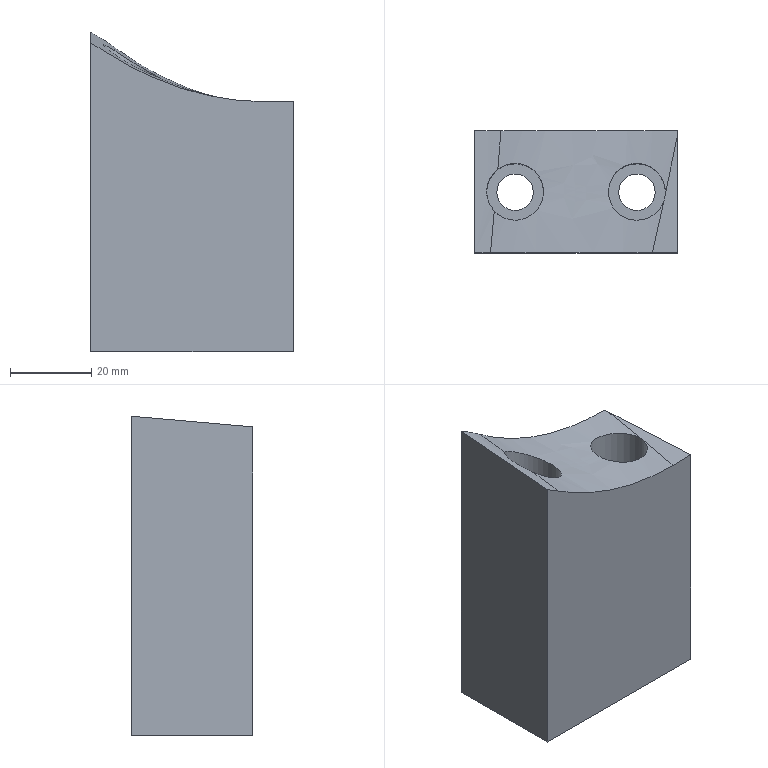Part | NX | features solid 2 | 1 solid | 14 faces | box 50.002 x 30 x 78.739 mm | volume 80442 mm3 | plane 7 | cylinder 4 | spline 3 | commonest cylinder face diameters 9 x2 14 x2
STEP:
#1=CARTESIAN_POINT('',(157.5,150.,-6.261));
#2=VERTEX_POINT('',#1);
#3=CARTESIAN_POINT('',(157.5,150.,-85.));
#4=VERTEX_POINT('',#3);
#5=CARTESIAN_POINT('',(157.5,150.,10.));
#6=DIRECTION('',(0.,0.,-1.));
#7=VECTOR('',#6,1000.);
#8=LINE('',#5,#7);
#9=EDGE_CURVE('',#2,#4,#8,.T.);
#10=ORIENTED_EDGE('',*,*,#9,.F.);
#11=CARTESIAN_POINT('',(164.005,150.,-10.429));
#12=VERTEX_POINT('',#11);
#13=CARTESIAN_POINT('',(157.5,150.,-6.261));
#14=CARTESIAN_POINT('',(159.786,150.,-7.489));
#15=CARTESIAN_POINT('',(161.955,150.,-8.881));
#16=CARTESIAN_POINT('',(164.008,150.,-10.435));
#17=B_SPLINE_CURVE_WITH_KNOTS('',3,(#13,#14,#15,#16),.UNSPECIFIED.,.F.,.F.,(4,4),(0.,0.007722),.UNSPECIFIED.);
#18=EDGE_CURVE('',#2,#12,#17,.T.);
#19=ORIENTED_EDGE('',*,*,#18,.T.);
#20=CARTESIAN_POINT('',(207.5,150.,-24.818));
#21=VERTEX_POINT('',#20);
#22=CARTESIAN_POINT('',(164.004,150.,-10.427));
#23=CARTESIAN_POINT('',(165.563,150.,-11.606));
#24=CARTESIAN_POINT('',(168.794,150.,-13.755));
#25=CARTESIAN_POINT('',(175.477,150.,-17.617));
#26=CARTESIAN_POINT('',(187.998,150.,-22.995));
#27=CARTESIAN_POINT('',(199.69,150.,-24.897));
#28=CARTESIAN_POINT('',(207.5,150.,-24.818));
#29=B_SPLINE_CURVE_WITH_KNOTS('',3,(#22,#23,#24,#25,#26,#27,#28),.UNSPECIFIED.,.F.,.F.,(4,1,1,1,4),(0.,0.00579,0.01158,0.02316,0.04632),.UNSPECIFIED.);
#30=EDGE_CURVE('',#12,#21,#29,.T.);
#31=ORIENTED_EDGE('',*,*,#30,.T.);
#32=CARTESIAN_POINT('',(207.5,150.,-85.));
#33=VERTEX_POINT('',#32);
#34=CARTESIAN_POINT('',(207.5,150.,10.));
#35=DIRECTION('',(0.,0.,-1.));
#36=VECTOR('',#35,1000.);
#37=LINE('',#34,#36);
#38=EDGE_CURVE('',#21,#33,#37,.T.);
#39=ORIENTED_EDGE('',*,*,#38,.T.);
#40=CARTESIAN_POINT('',(157.5,150.,-85.));
#41=DIRECTION('',(1.,0.,0.));
#42=VECTOR('',#41,1000.);
#43=LINE('',#40,#42);
#44=EDGE_CURVE('',#4,#33,#43,.T.);
#45=ORIENTED_EDGE('',*,*,#44,.F.);
#46=EDGE_LOOP('',(#10,#19,#31,#39,#45));
#47=FACE_BOUND('',#46,.T.);
#48=CARTESIAN_POINT('',(157.5,150.,10.));
#49=DIRECTION('',(0.,-1.,0.));
#50=DIRECTION('',(0.,0.,-1.));
#51=AXIS2_PLACEMENT_3D('',#48,#49,#50);
#52=PLANE('',#51);
#53=ADVANCED_FACE('',(#47),#52,.F.);
#54=CARTESIAN_POINT('',(207.5,120.,-23.313));
#55=VERTEX_POINT('',#54);
#56=CARTESIAN_POINT('',(207.5,120.,-85.));
#57=VERTEX_POINT('',#56);
#58=CARTESIAN_POINT('',(207.5,120.,10.));
#59=DIRECTION('',(0.,0.,-1.));
#60=VECTOR('',#59,1000.);
#61=LINE('',#58,#60);
#62=EDGE_CURVE('',#55,#57,#61,.T.);
#63=ORIENTED_EDGE('',*,*,#62,.F.);
#64=CARTESIAN_POINT('',(201.315,120.,-23.399));
#65=VERTEX_POINT('',#64);
#66=CARTESIAN_POINT('',(207.5,120.,-23.313));
#67=CARTESIAN_POINT('',(205.438,120.,-23.34));
#68=CARTESIAN_POINT('',(203.376,120.,-23.366));
#69=CARTESIAN_POINT('',(201.314,120.,-23.393));
#70=B_SPLINE_CURVE_WITH_KNOTS('',3,(#66,#67,#68,#69),.UNSPECIFIED.,.F.,.F.,(4,4),(0.,0.006187),.UNSPECIFIED.);
#71=EDGE_CURVE('',#55,#65,#70,.T.);
#72=ORIENTED_EDGE('',*,*,#71,.T.);
#73=CARTESIAN_POINT('',(161.435,120.,-11.237));
#74=VERTEX_POINT('',#73);
#75=CARTESIAN_POINT('',(201.315,120.,-23.401));
#76=CARTESIAN_POINT('',(194.24,120.,-23.492));
#77=CARTESIAN_POINT('',(183.7,120.,-21.839));
#78=CARTESIAN_POINT('',(172.184,120.,-17.245));
#79=CARTESIAN_POINT('',(165.954,120.,-13.988));
#80=CARTESIAN_POINT('',(162.91,120.,-12.213));
#81=CARTESIAN_POINT('',(161.434,120.,-11.237));
#82=B_SPLINE_CURVE_WITH_KNOTS('',3,(#75,#76,#77,#78,#79,#80,#81),.UNSPECIFIED.,.F.,.F.,(4,1,1,1,4),(0.,0.02111,0.03166,0.03694,0.04222),.UNSPECIFIED.);
#83=EDGE_CURVE('',#65,#74,#82,.T.);
#84=ORIENTED_EDGE('',*,*,#83,.T.);
#85=CARTESIAN_POINT('',(157.5,120.,-8.886));
#86=VERTEX_POINT('',#85);
#87=CARTESIAN_POINT('',(161.436,120.,-11.238));
#88=CARTESIAN_POINT('',(160.164,120.,-10.397));
#89=CARTESIAN_POINT('',(158.853,120.,-9.613));
#90=CARTESIAN_POINT('',(157.5,120.,-8.886));
#91=B_SPLINE_CURVE_WITH_KNOTS('',3,(#87,#88,#89,#90),.UNSPECIFIED.,.F.,.F.,(4,4),(0.008039,0.01261),.UNSPECIFIED.);
#92=EDGE_CURVE('',#74,#86,#91,.T.);
#93=ORIENTED_EDGE('',*,*,#92,.T.);
#94=CARTESIAN_POINT('',(157.5,120.,-85.));
#95=VERTEX_POINT('',#94);
#96=CARTESIAN_POINT('',(157.5,120.,10.));
#97=DIRECTION('',(0.,0.,-1.));
#98=VECTOR('',#97,1000.);
#99=LINE('',#96,#98);
#100=EDGE_CURVE('',#86,#95,#99,.T.);
#101=ORIENTED_EDGE('',*,*,#100,.T.);
#102=CARTESIAN_POINT('',(157.5,120.,-85.));
#103=DIRECTION('',(-1.,0.,0.));
#104=VECTOR('',#103,1000.);
#105=LINE('',#102,#104);
#106=EDGE_CURVE('',#95,#57,#105,.F.);
#107=ORIENTED_EDGE('',*,*,#106,.T.);
#108=EDGE_LOOP('',(#63,#72,#84,#93,#101,#107));
#109=FACE_BOUND('',#108,.T.);
#110=CARTESIAN_POINT('',(157.5,120.,10.));
#111=DIRECTION('',(0.,-1.,0.));
#112=DIRECTION('',(0.,0.,-1.));
#113=AXIS2_PLACEMENT_3D('',#110,#111,#112);
#114=PLANE('',#113);
#115=ADVANCED_FACE('',(#109),#114,.T.);
#116=CARTESIAN_POINT('',(207.5,148.88,-24.761));
#117=VERTEX_POINT('',#116);
#118=CARTESIAN_POINT('',(207.5,120.,-23.313));
#119=CARTESIAN_POINT('',(207.5,129.639,-23.784));
#120=CARTESIAN_POINT('',(207.5,139.278,-24.27));
#121=CARTESIAN_POINT('',(207.5,148.916,-24.759));
#122=B_SPLINE_CURVE_WITH_KNOTS('',3,(#118,#119,#120,#121),.UNSPECIFIED.,.F.,.F.,(4,4),(0.,0.02895),.UNSPECIFIED.);
#123=EDGE_CURVE('',#55,#117,#122,.T.);
#124=ORIENTED_EDGE('',*,*,#123,.F.);
#125=ORIENTED_EDGE('',*,*,#62,.T.);
#126=CARTESIAN_POINT('',(207.5,150.,-85.));
#127=DIRECTION('',(0.,1.,0.));
#128=VECTOR('',#127,1000.);
#129=LINE('',#126,#128);
#130=EDGE_CURVE('',#33,#57,#129,.F.);
#131=ORIENTED_EDGE('',*,*,#130,.F.);
#132=ORIENTED_EDGE('',*,*,#38,.F.);
#133=CARTESIAN_POINT('',(207.5,148.868,-24.761));
#134=CARTESIAN_POINT('',(207.5,149.246,-24.78));
#135=CARTESIAN_POINT('',(207.5,149.623,-24.799));
#136=CARTESIAN_POINT('',(207.5,150.,-24.818));
#137=B_SPLINE_CURVE_WITH_KNOTS('',3,(#133,#134,#135,#136),.UNSPECIFIED.,.F.,.F.,(4,4),(0.,0.001133),.UNSPECIFIED.);
#138=EDGE_CURVE('',#117,#21,#137,.T.);
#139=ORIENTED_EDGE('',*,*,#138,.F.);
#140=EDGE_LOOP('',(#124,#125,#131,#132,#139));
#141=FACE_BOUND('',#140,.T.);
#142=CARTESIAN_POINT('',(207.5,150.,10.));
#143=DIRECTION('',(-1.,0.,0.));
#144=DIRECTION('',(0.,0.,-1.));
#145=AXIS2_PLACEMENT_3D('',#142,#143,#144);
#146=PLANE('',#145);
#147=ADVANCED_FACE('',(#141),#146,.F.);
#148=ORIENTED_EDGE('',*,*,#100,.F.);
#149=CARTESIAN_POINT('',(157.5,120.,-8.886));
#150=CARTESIAN_POINT('',(157.5,130.,-8.011));
#151=CARTESIAN_POINT('',(157.5,140.,-7.136));
#152=CARTESIAN_POINT('',(157.5,150.,-6.261));
#153=B_SPLINE_CURVE_WITH_KNOTS('',3,(#149,#150,#151,#152),.UNSPECIFIED.,.F.,.F.,(4,4),(0.,0.03011),.UNSPECIFIED.);
#154=EDGE_CURVE('',#86,#2,#153,.T.);
#155=ORIENTED_EDGE('',*,*,#154,.T.);
#156=ORIENTED_EDGE('',*,*,#9,.T.);
#157=CARTESIAN_POINT('',(157.5,150.,-85.));
#158=DIRECTION('',(0.,1.,0.));
#159=VECTOR('',#158,1000.);
#160=LINE('',#157,#159);
#161=EDGE_CURVE('',#4,#95,#160,.F.);
#162=ORIENTED_EDGE('',*,*,#161,.T.);
#163=EDGE_LOOP('',(#148,#155,#156,#162));
#164=FACE_BOUND('',#163,.T.);
#165=CARTESIAN_POINT('',(157.5,150.,10.));
#166=DIRECTION('',(-1.,0.,0.));
#167=DIRECTION('',(0.,0.,-1.));
#168=AXIS2_PLACEMENT_3D('',#165,#166,#167);
#169=PLANE('',#168);
#170=ADVANCED_FACE('',(#164),#169,.T.);
#171=CARTESIAN_POINT('',(160.5,135.,-75.));
#172=VERTEX_POINT('',#171);
#173=CARTESIAN_POINT('',(167.5,135.,-75.));
#174=DIRECTION('',(0.,0.,-1.));
#175=DIRECTION('',(-1.,0.,0.));
#176=AXIS2_PLACEMENT_3D('',#173,#174,#175);
#177=CIRCLE('',#176,7.);
#178=EDGE_CURVE('',#172,#172,#177,.F.);
#179=ORIENTED_EDGE('',*,*,#178,.F.);
#180=EDGE_LOOP('',(#179));
#181=FACE_BOUND('',#180,.T.);
#182=CARTESIAN_POINT('',(162.356,130.252,-10.963));
#183=VERTEX_POINT('',#182);
#184=CARTESIAN_POINT('',(163.237,140.552,-10.687));
#185=VERTEX_POINT('',#184);
#186=CARTESIAN_POINT('',(162.357,130.251,-10.966));
#187=CARTESIAN_POINT('',(161.754,130.905,-10.49));
#188=CARTESIAN_POINT('',(160.736,132.517,-9.683));
#189=CARTESIAN_POINT('',(160.293,135.562,-9.143));
#190=CARTESIAN_POINT('',(161.226,138.566,-9.463));
#191=CARTESIAN_POINT('',(162.526,140.007,-10.22));
#192=CARTESIAN_POINT('',(163.239,140.554,-10.691));
#193=B_SPLINE_CURVE_WITH_KNOTS('',3,(#186,#187,#188,#189,#190,#191,#192),.UNSPECIFIED.,.F.,.F.,(4,1,1,1,4),(0.007546,0.01057,0.01359,0.01661,0.01963),.UNSPECIFIED.);
#194=EDGE_CURVE('',#183,#185,#193,.T.);
#195=ORIENTED_EDGE('',*,*,#194,.F.);
#196=CARTESIAN_POINT('',(163.236,140.552,-10.685));
#197=CARTESIAN_POINT('',(164.285,141.357,-11.377));
#198=CARTESIAN_POINT('',(166.693,142.286,-12.911));
#199=CARTESIAN_POINT('',(170.543,141.711,-15.262));
#200=CARTESIAN_POINT('',(173.799,138.976,-17.068));
#201=CARTESIAN_POINT('',(174.982,134.474,-17.772));
#202=CARTESIAN_POINT('',(173.168,130.15,-17.123));
#203=CARTESIAN_POINT('',(169.484,127.887,-15.43));
#204=CARTESIAN_POINT('',(165.492,127.934,-13.177));
#205=CARTESIAN_POINT('',(163.249,129.284,-11.667));
#206=CARTESIAN_POINT('',(162.356,130.252,-10.962));
#207=B_SPLINE_CURVE_WITH_KNOTS('',3,(#196,#197,#198,#199,#200,#201,#202,#203,#204,#205,#206),.UNSPECIFIED.,.F.,.F.,(4,1,1,1,1,1,1,1,4),(0.,0.004389,0.008779,0.01317,0.01756,0.02195,0.02634,0.03072,0.03511),.UNSPECIFIED.);
#208=EDGE_CURVE('',#185,#183,#207,.T.);
#209=ORIENTED_EDGE('',*,*,#208,.F.);
#210=EDGE_LOOP('',(#195,#209));
#211=FACE_BOUND('',#210,.T.);
#212=CARTESIAN_POINT('',(167.5,135.,10.));
#213=DIRECTION('',(0.,0.,-1.));
#214=DIRECTION('',(1.,0.,0.));
#215=AXIS2_PLACEMENT_3D('',#212,#213,#214);
#216=CYLINDRICAL_SURFACE('',#215,7.);
#217=ADVANCED_FACE('',(#181,#211),#216,.F.);
#218=CARTESIAN_POINT('',(202.,135.,-85.));
#219=VERTEX_POINT('',#218);
#220=CARTESIAN_POINT('',(197.5,135.,-85.));
#221=DIRECTION('',(0.,0.,1.));
#222=DIRECTION('',(1.,0.,0.));
#223=AXIS2_PLACEMENT_3D('',#220,#221,#222);
#224=CIRCLE('',#223,4.5);
#225=EDGE_CURVE('',#219,#219,#224,.T.);
#226=ORIENTED_EDGE('',*,*,#225,.T.);
#227=EDGE_LOOP('',(#226));
#228=FACE_BOUND('',#227,.T.);
#229=CARTESIAN_POINT('',(172.,135.,-85.));
#230=VERTEX_POINT('',#229);
#231=CARTESIAN_POINT('',(167.5,135.,-85.));
#232=DIRECTION('',(0.,0.,1.));
#233=DIRECTION('',(1.,0.,0.));
#234=AXIS2_PLACEMENT_3D('',#231,#232,#233);
#235=CIRCLE('',#234,4.5);
#236=EDGE_CURVE('',#230,#230,#235,.T.);
#237=ORIENTED_EDGE('',*,*,#236,.T.);
#238=EDGE_LOOP('',(#237));
#239=FACE_BOUND('',#238,.T.);
#240=ORIENTED_EDGE('',*,*,#44,.T.);
#241=ORIENTED_EDGE('',*,*,#130,.T.);
#242=ORIENTED_EDGE('',*,*,#106,.F.);
#243=ORIENTED_EDGE('',*,*,#161,.F.);
#244=EDGE_LOOP('',(#240,#241,#242,#243));
#245=FACE_BOUND('',#244,.T.);
#246=CARTESIAN_POINT('',(157.5,150.,-85.));
#247=DIRECTION('',(0.,0.,1.));
#248=DIRECTION('',(0.,-1.,0.));
#249=AXIS2_PLACEMENT_3D('',#246,#247,#248);
#250=PLANE('',#249);
#251=ADVANCED_FACE('',(#228,#239,#245),#250,.F.);
#252=ORIENTED_EDGE('',*,*,#236,.F.);
#253=EDGE_LOOP('',(#252));
#254=FACE_BOUND('',#253,.T.);
#255=CARTESIAN_POINT('',(163.,135.,-75.));
#256=VERTEX_POINT('',#255);
#257=CARTESIAN_POINT('',(167.5,135.,-75.));
#258=DIRECTION('',(0.,0.,-1.));
#259=DIRECTION('',(-1.,0.,0.));
#260=AXIS2_PLACEMENT_3D('',#257,#258,#259);
#261=CIRCLE('',#260,4.5);
#262=EDGE_CURVE('',#256,#256,#261,.F.);
#263=ORIENTED_EDGE('',*,*,#262,.T.);
#264=EDGE_LOOP('',(#263));
#265=FACE_BOUND('',#264,.T.);
#266=CARTESIAN_POINT('',(167.5,135.,-140.));
#267=DIRECTION('',(0.,0.,-1.));
#268=DIRECTION('',(1.,0.,0.));
#269=AXIS2_PLACEMENT_3D('',#266,#267,#268);
#270=CYLINDRICAL_SURFACE('',#269,4.5);
#271=ADVANCED_FACE('',(#254,#265),#270,.F.);
#272=ORIENTED_EDGE('',*,*,#262,.F.);
#273=EDGE_LOOP('',(#272));
#274=FACE_BOUND('',#273,.T.);
#275=ORIENTED_EDGE('',*,*,#178,.T.);
#276=EDGE_LOOP('',(#275));
#277=FACE_BOUND('',#276,.T.);
#278=CARTESIAN_POINT('',(167.5,135.,-75.));
#279=DIRECTION('',(0.,0.,-1.));
#280=DIRECTION('',(1.,0.,0.));
#281=AXIS2_PLACEMENT_3D('',#278,#279,#280);
#282=PLANE('',#281);
#283=ADVANCED_FACE('',(#274,#277),#282,.F.);
#284=ORIENTED_EDGE('',*,*,#225,.F.);
#285=EDGE_LOOP('',(#284));
#286=FACE_BOUND('',#285,.T.);
#287=CARTESIAN_POINT('',(193.,135.,-75.));
#288=VERTEX_POINT('',#287);
#289=CARTESIAN_POINT('',(197.5,135.,-75.));
#290=DIRECTION('',(0.,0.,-1.));
#291=DIRECTION('',(-1.,0.,0.));
#292=AXIS2_PLACEMENT_3D('',#289,#290,#291);
#293=CIRCLE('',#292,4.5);
#294=EDGE_CURVE('',#288,#288,#293,.F.);
#295=ORIENTED_EDGE('',*,*,#294,.T.);
#296=EDGE_LOOP('',(#295));
#297=FACE_BOUND('',#296,.T.);
#298=CARTESIAN_POINT('',(197.5,135.,-140.));
#299=DIRECTION('',(0.,0.,-1.));
#300=DIRECTION('',(1.,0.,0.));
#301=AXIS2_PLACEMENT_3D('',#298,#299,#300);
#302=CYLINDRICAL_SURFACE('',#301,4.5);
#303=ADVANCED_FACE('',(#286,#297),#302,.F.);
#304=ORIENTED_EDGE('',*,*,#294,.F.);
#305=EDGE_LOOP('',(#304));
#306=FACE_BOUND('',#305,.T.);
#307=CARTESIAN_POINT('',(190.5,135.,-75.));
#308=VERTEX_POINT('',#307);
#309=CARTESIAN_POINT('',(197.5,135.,-75.));
#310=DIRECTION('',(0.,0.,-1.));
#311=DIRECTION('',(-1.,0.,0.));
#312=AXIS2_PLACEMENT_3D('',#309,#310,#311);
#313=CIRCLE('',#312,7.);
#314=EDGE_CURVE('',#308,#308,#313,.F.);
#315=ORIENTED_EDGE('',*,*,#314,.T.);
#316=EDGE_LOOP('',(#315));
#317=FACE_BOUND('',#316,.T.);
#318=CARTESIAN_POINT('',(197.5,135.,-75.));
#319=DIRECTION('',(0.,0.,-1.));
#320=DIRECTION('',(1.,0.,0.));
#321=AXIS2_PLACEMENT_3D('',#318,#319,#320);
#322=PLANE('',#321);
#323=ADVANCED_FACE('',(#306,#317),#322,.F.);
#324=CARTESIAN_POINT('',(204.192,132.956,-24.001));
#325=VERTEX_POINT('',#324);
#326=CARTESIAN_POINT('',(204.44,134.108,-24.055));
#327=VERTEX_POINT('',#326);
#328=CARTESIAN_POINT('',(204.195,132.956,-24.004));
#329=CARTESIAN_POINT('',(203.668,131.23,-23.925));
#330=CARTESIAN_POINT('',(201.254,128.262,-23.829));
#331=CARTESIAN_POINT('',(195.538,127.541,-23.511));
#332=CARTESIAN_POINT('',(190.93,130.952,-22.865));
#333=CARTESIAN_POINT('',(189.961,136.658,-22.677));
#334=CARTESIAN_POINT('',(193.196,141.387,-23.404));
#335=CARTESIAN_POINT('',(198.761,142.61,-24.236));
#336=CARTESIAN_POINT('',(203.698,139.598,-24.363));
#337=CARTESIAN_POINT('',(204.673,135.897,-24.145));
#338=CARTESIAN_POINT('',(204.443,134.107,-24.058));
#339=B_SPLINE_CURVE_WITH_KNOTS('',3,(#328,#329,#330,#331,#332,#333,#334,#335,#336,#337,#338),.UNSPECIFIED.,.F.,.F.,(4,1,1,1,1,1,1,1,4),(0.,0.005342,0.01068,0.01602,0.02137,0.02671,0.03205,0.03739,0.04273),.UNSPECIFIED.);
#340=EDGE_CURVE('',#325,#327,#339,.T.);
#341=ORIENTED_EDGE('',*,*,#340,.F.);
#342=CARTESIAN_POINT('',(204.328,133.532,-24.026));
#343=VERTEX_POINT('',#342);
#344=CARTESIAN_POINT('',(204.195,132.956,-24.004));
#345=CARTESIAN_POINT('',(204.252,133.144,-24.013));
#346=CARTESIAN_POINT('',(204.302,133.335,-24.022));
#347=CARTESIAN_POINT('',(204.344,133.528,-24.031));
#348=B_SPLINE_CURVE_WITH_KNOTS('',3,(#344,#345,#346,#347),.UNSPECIFIED.,.F.,.F.,(4,4),(0.,1.),.UNSPECIFIED.);
#349=EDGE_CURVE('',#325,#343,#348,.T.);
#350=ORIENTED_EDGE('',*,*,#349,.T.);
#351=CARTESIAN_POINT('',(204.344,133.528,-24.031));
#352=CARTESIAN_POINT('',(204.385,133.72,-24.04));
#353=CARTESIAN_POINT('',(204.418,133.913,-24.049));
#354=CARTESIAN_POINT('',(204.443,134.107,-24.058));
#355=B_SPLINE_CURVE_WITH_KNOTS('',3,(#351,#352,#353,#354),.UNSPECIFIED.,.F.,.F.,(4,4),(0.,1.),.UNSPECIFIED.);
#356=EDGE_CURVE('',#343,#327,#355,.T.);
#357=ORIENTED_EDGE('',*,*,#356,.T.);
#358=EDGE_LOOP('',(#341,#350,#357));
#359=FACE_BOUND('',#358,.T.);
#360=ORIENTED_EDGE('',*,*,#314,.F.);
#361=EDGE_LOOP('',(#360));
#362=FACE_BOUND('',#361,.T.);
#363=CARTESIAN_POINT('',(197.5,135.,10.));
#364=DIRECTION('',(0.,0.,-1.));
#365=DIRECTION('',(1.,0.,0.));
#366=AXIS2_PLACEMENT_3D('',#363,#364,#365);
#367=CYLINDRICAL_SURFACE('',#366,7.);
#368=ADVANCED_FACE('',(#359,#362),#367,.F.);
#369=ORIENTED_EDGE('',*,*,#18,.F.);
#370=ORIENTED_EDGE('',*,*,#154,.F.);
#371=ORIENTED_EDGE('',*,*,#92,.F.);
#372=CARTESIAN_POINT('',(161.436,120.,-11.238));
#373=CARTESIAN_POINT('',(161.452,120.172,-11.234));
#374=CARTESIAN_POINT('',(161.476,120.442,-11.226));
#375=CARTESIAN_POINT('',(161.505,120.755,-11.218));
#376=CARTESIAN_POINT('',(161.569,121.458,-11.199));
#377=CARTESIAN_POINT('',(161.696,122.842,-11.163));
#378=CARTESIAN_POINT('',(161.976,125.936,-11.08));
#379=CARTESIAN_POINT('',(162.206,128.525,-11.012));
#380=CARTESIAN_POINT('',(162.357,130.252,-10.966));
#381=B_SPLINE_CURVE_WITH_KNOTS('',3,(#372,#373,#374,#375,#376,#377,#378,#379,#380),.UNSPECIFIED.,.F.,.F.,(4,1,1,1,1,1,4),(0.7471,0.749,0.75,0.751,0.7548,0.7625,0.7778),.UNSPECIFIED.);
#382=EDGE_CURVE('',#74,#183,#381,.T.);
#383=ORIENTED_EDGE('',*,*,#382,.T.);
#384=ORIENTED_EDGE('',*,*,#194,.T.);
#385=CARTESIAN_POINT('',(163.239,140.553,-10.691));
#386=CARTESIAN_POINT('',(163.505,143.734,-10.605));
#387=CARTESIAN_POINT('',(163.761,146.883,-10.52));
#388=CARTESIAN_POINT('',(164.008,150.,-10.435));
#389=B_SPLINE_CURVE_WITH_KNOTS('',3,(#385,#386,#387,#388),.UNSPECIFIED.,.F.,.F.,(4,4),(0.8086,0.8375),.UNSPECIFIED.);
#390=EDGE_CURVE('',#185,#12,#389,.T.);
#391=ORIENTED_EDGE('',*,*,#390,.T.);
#392=EDGE_LOOP('',(#369,#370,#371,#383,#384,#391));
#393=FACE_BOUND('',#392,.T.);
#394=CARTESIAN_POINT('',(164.045,119.979,-13.089));
#395=CARTESIAN_POINT('',(160.916,119.773,-10.736));
#396=CARTESIAN_POINT('',(157.458,119.613,-8.898));
#397=CARTESIAN_POINT('',(164.045,127.41,-12.439));
#398=CARTESIAN_POINT('',(160.916,127.204,-10.086));
#399=CARTESIAN_POINT('',(157.458,127.044,-8.248));
#400=CARTESIAN_POINT('',(164.045,134.841,-11.789));
#401=CARTESIAN_POINT('',(160.917,134.635,-9.436));
#402=CARTESIAN_POINT('',(157.459,134.475,-7.597));
#403=CARTESIAN_POINT('',(164.045,145.03,-10.897));
#404=CARTESIAN_POINT('',(160.917,144.824,-8.544));
#405=CARTESIAN_POINT('',(157.459,144.663,-6.706));
#406=CARTESIAN_POINT('',(164.045,147.788,-10.656));
#407=CARTESIAN_POINT('',(160.917,147.582,-8.303));
#408=CARTESIAN_POINT('',(157.459,147.421,-6.465));
#409=CARTESIAN_POINT('',(164.045,150.546,-10.415));
#410=CARTESIAN_POINT('',(160.917,150.34,-8.062));
#411=CARTESIAN_POINT('',(157.459,150.179,-6.223));
#412=(BOUNDED_SURFACE()B_SPLINE_SURFACE(3,2,((#394,#395,#396),(#397,#398,#399),(#400,#401,#402),(#403,#404,#405),(#406,#407,#408),(#409,#410,#411)),.UNSPECIFIED.,.F.,.F.,.F.)B_SPLINE_SURFACE_WITH_KNOTS((4,2,4),(3,3),(0.829,0.875,0.8921),(0.2573,0.4329),.UNSPECIFIED.)GEOMETRIC_REPRESENTATION_ITEM()RATIONAL_B_SPLINE_SURFACE(((0.9635,0.9554,0.9531),(0.9635,0.9554,0.9531),(0.9635,0.9554,0.9531),(0.9635,0.9554,0.9531),(0.9635,0.9554,0.9531),(0.9635,0.9554,0.9531)))REPRESENTATION_ITEM('')SURFACE());
#413=ADVANCED_FACE('',(#393),#412,.T.);
#414=ORIENTED_EDGE('',*,*,#83,.F.);
#415=CARTESIAN_POINT('',(201.315,120.,-23.401));
#416=CARTESIAN_POINT('',(202.301,124.313,-23.598));
#417=CARTESIAN_POINT('',(203.261,128.631,-23.8));
#418=CARTESIAN_POINT('',(204.195,132.956,-24.004));
#419=B_SPLINE_CURVE_WITH_KNOTS('',3,(#415,#416,#417,#418),.UNSPECIFIED.,.F.,.F.,(4,4),(0.7682,0.8082),.UNSPECIFIED.);
#420=EDGE_CURVE('',#65,#325,#419,.T.);
#421=ORIENTED_EDGE('',*,*,#420,.T.);
#422=ORIENTED_EDGE('',*,*,#340,.T.);
#423=CARTESIAN_POINT('',(204.443,134.107,-24.058));
#424=CARTESIAN_POINT('',(205.5,139.028,-24.291));
#425=CARTESIAN_POINT('',(206.521,143.956,-24.526));
#426=CARTESIAN_POINT('',(207.505,148.891,-24.763));
#427=B_SPLINE_CURVE_WITH_KNOTS('',3,(#423,#424,#425,#426),.UNSPECIFIED.,.F.,.F.,(4,4),(0.8118,0.8573),.UNSPECIFIED.);
#428=EDGE_CURVE('',#327,#117,#427,.T.);
#429=ORIENTED_EDGE('',*,*,#428,.T.);
#430=ORIENTED_EDGE('',*,*,#138,.T.);
#431=ORIENTED_EDGE('',*,*,#30,.F.);
#432=ORIENTED_EDGE('',*,*,#390,.F.);
#433=ORIENTED_EDGE('',*,*,#208,.T.);
#434=ORIENTED_EDGE('',*,*,#382,.F.);
#435=EDGE_LOOP('',(#414,#421,#422,#429,#430,#431,#432,#433,#434));
#436=FACE_BOUND('',#435,.T.);
#437=CARTESIAN_POINT('',(199.739,113.193,-23.091));
#438=CARTESIAN_POINT('',(192.766,114.279,-23.233));
#439=CARTESIAN_POINT('',(184.266,115.67,-21.834));
#440=CARTESIAN_POINT('',(174.734,117.325,-18.346));
#441=CARTESIAN_POINT('',(170.12,118.149,-16.273));
#442=CARTESIAN_POINT('',(166.409,118.831,-14.302));
#443=CARTESIAN_POINT('',(163.884,119.305,-12.809));
#444=CARTESIAN_POINT('',(162.467,119.575,-11.921));
#445=CARTESIAN_POINT('',(161.759,119.71,-11.477));
#446=CARTESIAN_POINT('',(161.414,119.777,-11.243));
#447=CARTESIAN_POINT('',(199.813,113.505,-23.105));
#448=CARTESIAN_POINT('',(192.832,114.592,-23.248));
#449=CARTESIAN_POINT('',(184.32,115.984,-21.847));
#450=CARTESIAN_POINT('',(174.777,117.641,-18.353));
#451=CARTESIAN_POINT('',(170.158,118.466,-16.276));
#452=CARTESIAN_POINT('',(166.443,119.148,-14.3));
#453=CARTESIAN_POINT('',(163.916,119.623,-12.804));
#454=CARTESIAN_POINT('',(162.497,119.893,-11.914));
#455=CARTESIAN_POINT('',(161.789,120.028,-11.469));
#456=CARTESIAN_POINT('',(161.443,120.095,-11.234));
#457=CARTESIAN_POINT('',(202.69,125.792,-23.659));
#458=CARTESIAN_POINT('',(195.394,126.919,-23.81));
#459=CARTESIAN_POINT('',(186.453,128.37,-22.352));
#460=CARTESIAN_POINT('',(176.466,130.095,-18.615));
#461=CARTESIAN_POINT('',(171.641,130.952,-16.381));
#462=CARTESIAN_POINT('',(167.774,131.659,-14.241));
#463=CARTESIAN_POINT('',(165.154,132.149,-12.613));
#464=CARTESIAN_POINT('',(163.686,132.427,-11.642));
#465=CARTESIAN_POINT('',(162.953,132.566,-11.154));
#466=CARTESIAN_POINT('',(162.597,132.635,-10.898));
#467=CARTESIAN_POINT('',(205.376,138.123,-24.246));
#468=CARTESIAN_POINT('',(197.78,139.283,-24.405));
#469=CARTESIAN_POINT('',(188.423,140.786,-22.886));
#470=CARTESIAN_POINT('',(178.011,142.571,-18.898));
#471=CARTESIAN_POINT('',(172.993,143.457,-16.5));
#472=CARTESIAN_POINT('',(168.986,144.184,-14.193));
#473=CARTESIAN_POINT('',(166.281,144.687,-12.428));
#474=CARTESIAN_POINT('',(164.769,144.972,-11.375));
#475=CARTESIAN_POINT('',(164.016,145.114,-10.843));
#476=CARTESIAN_POINT('',(163.65,145.185,-10.566));
#477=CARTESIAN_POINT('',(207.762,150.187,-24.825));
#478=CARTESIAN_POINT('',(199.896,151.372,-24.989));
#479=CARTESIAN_POINT('',(190.163,152.918,-23.401));
#480=CARTESIAN_POINT('',(179.369,154.751,-19.158));
#481=CARTESIAN_POINT('',(174.179,155.659,-16.598));
#482=CARTESIAN_POINT('',(170.049,156.403,-14.123));
#483=CARTESIAN_POINT('',(167.273,156.916,-12.226));
#484=CARTESIAN_POINT('',(165.724,157.206,-11.092));
#485=CARTESIAN_POINT('',(164.955,157.351,-10.518));
#486=CARTESIAN_POINT('',(164.58,157.422,-10.22));
#487=B_SPLINE_SURFACE_WITH_KNOTS('',3,3,((#437,#438,#439,#440,#441,#442,#443,#444,#445,#446),(#447,#448,#449,#450,#451,#452,#453,#454,#455,#456),(#457,#458,#459,#460,#461,#462,#463,#464,#465,#466),(#467,#468,#469,#470,#471,#472,#473,#474,#475,#476),(#477,#478,#479,#480,#481,#482,#483,#484,#485,#486)),.UNSPECIFIED.,.F.,.F.,.F.,(4,1,4),(4,1,1,1,1,1,1,4),(0.7471,0.75,0.8613),(0.,0.5,0.625,0.75,0.875,0.9375,0.9688,1.),.UNSPECIFIED.);
#488=ADVANCED_FACE('',(#436),#487,.T.);
#489=ORIENTED_EDGE('',*,*,#71,.F.);
#490=ORIENTED_EDGE('',*,*,#123,.T.);
#491=ORIENTED_EDGE('',*,*,#428,.F.);
#492=ORIENTED_EDGE('',*,*,#356,.F.);
#493=ORIENTED_EDGE('',*,*,#349,.F.);
#494=ORIENTED_EDGE('',*,*,#420,.F.);
#495=EDGE_LOOP('',(#489,#490,#491,#492,#493,#494));
#496=FACE_BOUND('',#495,.T.);
#497=CARTESIAN_POINT('',(207.501,149.089,-24.768));
#498=CARTESIAN_POINT('',(208.616,149.089,-24.753));
#499=CARTESIAN_POINT('',(211.161,149.089,-24.719));
#500=CARTESIAN_POINT('',(213.707,149.089,-24.686));
#501=CARTESIAN_POINT('',(215.138,149.089,-24.668));
#502=CARTESIAN_POINT('',(204.882,139.337,-24.308));
#503=CARTESIAN_POINT('',(206.007,139.337,-24.293));
#504=CARTESIAN_POINT('',(208.577,139.337,-24.26));
#505=CARTESIAN_POINT('',(211.148,139.337,-24.226));
#506=CARTESIAN_POINT('',(212.593,139.337,-24.208));
#507=CARTESIAN_POINT('',(202.262,129.582,-23.849));
#508=CARTESIAN_POINT('',(203.398,129.582,-23.834));
#509=CARTESIAN_POINT('',(205.993,129.582,-23.801));
#510=CARTESIAN_POINT('',(208.588,129.582,-23.767));
#511=CARTESIAN_POINT('',(210.047,129.582,-23.748));
#512=CARTESIAN_POINT('',(199.643,119.826,-23.406));
#513=CARTESIAN_POINT('',(200.79,119.826,-23.391));
#514=CARTESIAN_POINT('',(203.409,119.826,-23.357));
#515=CARTESIAN_POINT('',(206.029,119.826,-23.324));
#516=CARTESIAN_POINT('',(207.501,119.826,-23.305));
#517=B_SPLINE_SURFACE_WITH_KNOTS('',3,3,((#497,#498,#499,#500,#501),(#502,#503,#504,#505,#506),(#507,#508,#509,#510,#511),(#512,#513,#514,#515,#516)),.UNSPECIFIED.,.F.,.F.,.F.,(4,4),(4,1,4),(0.2154,0.2989),(0.0173,0.02344,0.03132),.UNSPECIFIED.);
#518=ADVANCED_FACE('',(#496),#517,.T.);
#519=CLOSED_SHELL('',(#53,#115,#147,#170,#217,#251,#271,#283,#303,#323,#368,#413,#488,#518));
#520=MANIFOLD_SOLID_BREP('',#519);
#521=(LENGTH_UNIT()NAMED_UNIT(*)SI_UNIT(.MILLI.,.METRE.));
#522=UNCERTAINTY_MEASURE_WITH_UNIT(LENGTH_MEASURE(0.1822),#521,'','');
#523=(NAMED_UNIT(*)PLANE_ANGLE_UNIT()SI_UNIT($,.RADIAN.));
#524=(NAMED_UNIT(*)SI_UNIT($,.STERADIAN.)SOLID_ANGLE_UNIT());
#525=(GEOMETRIC_REPRESENTATION_CONTEXT(3)GLOBAL_UNCERTAINTY_ASSIGNED_CONTEXT((#522))GLOBAL_UNIT_ASSIGNED_CONTEXT((#521,#523,#524))REPRESENTATION_CONTEXT('',''));
#526=ADVANCED_BREP_SHAPE_REPRESENTATION('',(#520),#525);